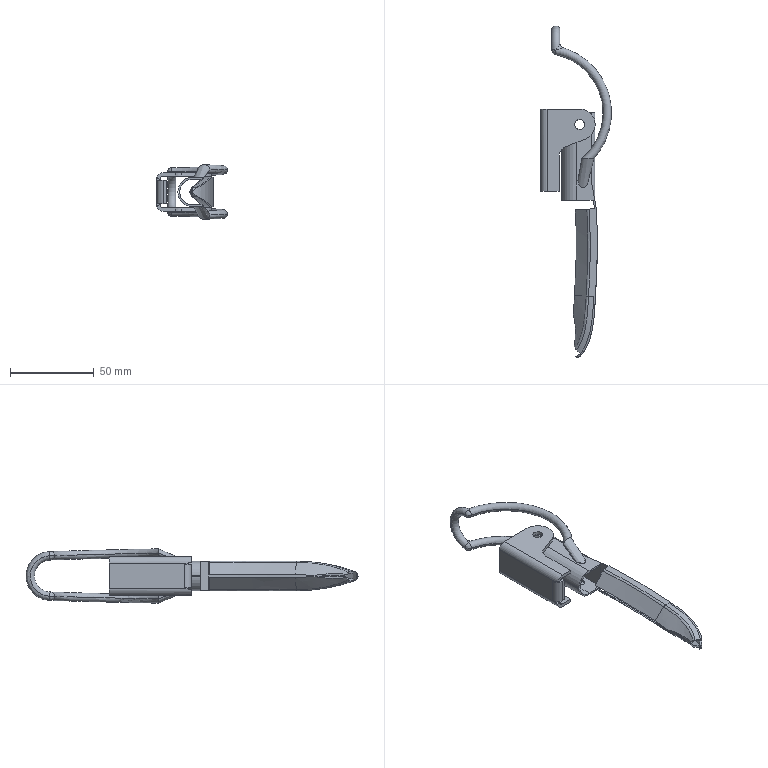Part | SolidWorks | 1 solid | 132 faces | box 42.182 x 197.75 x 32.336 mm | volume 16401 mm3 | plane 50 | cylinder 38 | spline 38 | torus 6 | commonest cylinder face diameters 6 x12 4 x5 204 x5 18.5 x4 8 x3 6.015 x2